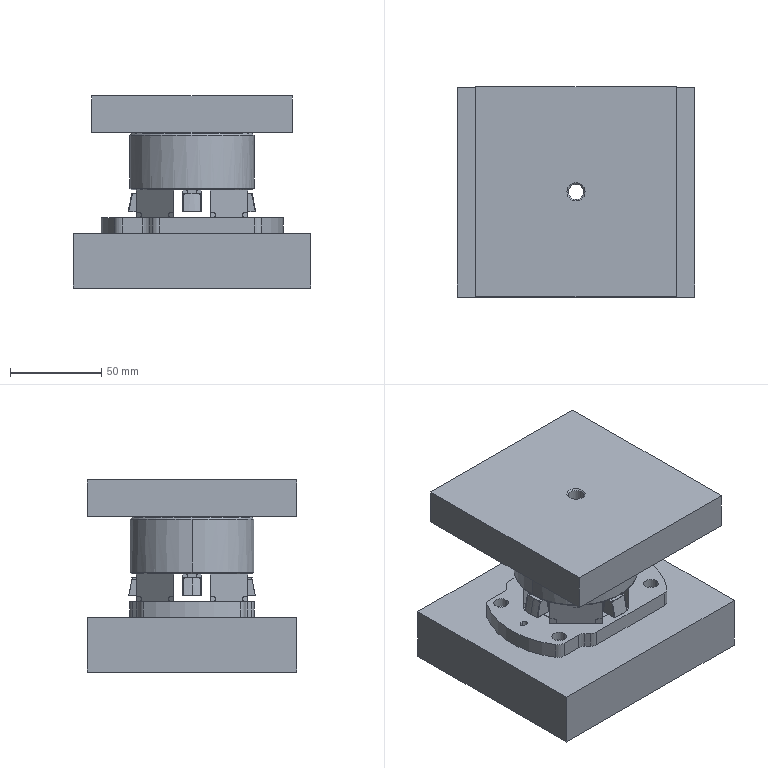CAM job | NX | 3+2 milling, drilling | part box 130 x 115 x 105.2 mm
Tools:
number,name,description,diameter,corner_radius,flute_length,length,flutes
12,ER16-D4-23,Milling Tool-5 Parameters,4.0,0.0,10.0,23.0,2
0,D1.5R0,Milling Tool-5 Parameters,1.5,0.0,50.0,75.0,2
20,D2,Milling Tool-5 Parameters,2.0,0.0,5.0,25.0,2
4,ER25-D10-50,Milling Tool-5 Parameters,10.0,0.0,20.0,50.0,2
11,ER25-D4-32,Milling Tool-5 Parameters,4.0,0.0,10.0,32.0,2
14,ER25-D2.5-23,Milling Tool-5 Parameters,2.5,0.0,0.0,10.0,2
16,ER25-D1.5-23,Milling Tool-5 Parameters,1.5,0.0,3.0,3.0,2
5,ER25-D10-50_G,Milling Tool-5 Parameters,10.0,0.0,20.0,50.0,2
12,ER25-D4-32_G,Milling Tool-5 Parameters,4.0,0.0,10.0,32.0,2
15,ER25-D2.5-23_G,Milling Tool-5 Parameters,2.5,0.0,10.0,10.0,2
17,ER25-D1.5-23_G,Milling Tool-5 Parameters,1.5,0.0,3.0,3.0,2
10,D8-55_PLUNGE,Milling Tool-5 Parameters,8.0,0.0,20.0,55.0,2
1,D50-120,Milling Tool-5 Parameters,50.0,0.0,5.0,120.0,2
3,D8.6,Drilling Tool,8.6,0.0,35.0,80.0,2
7,M4_D3.4,Drilling Tool,3.4,0.0,20.0,30.0,2
6,M10,Drilling Tool,8.6,0.0,35.0,40.0,2
8,M4,Drilling Tool,3.4,0.0,10.0,20.0,2
9,DRILL_D4.5,Drilling Tool,4.5,0.0,35.0,60.0,2
2,Φ10_CHAMFER,Chamfer Mill,10.0,0.0,20.0,55.0,2
Operations:
program,operation,operation_type,tool,method,geometry_group,spindle_rpm,surface_speed,feed_per_tooth,feed_cut,feed_plunge,cut_length_mm,path_length_mm,cut_time_min,machine_time_min
STEP1_FIXTURE,11,VolumeBased25DMillingOperation,D50-120,METHOD,MCS_1,3000.0,471.0,0.1667,1000.0,100.0,668.5,877.9,0.6685,0.6894
STEP1_FIXTURE,12,Operation,Φ10_CHAMFER,METHOD,MCS_1,2000.0,188.0,0.0125,100.0,100.0,16.0,462.529,0.16,0.2047
STEP1_FIXTURE,13,Operation,D8.6,METHOD,MCS_1,1400.0,37.0,0.0714,200.0,100.0,36.0,282.4,0.18,0.2046
STEP1_FIXTURE,14,PlanarMilling,ER25-D10-50,METHOD,MCS_1,5000.0,157.0,0.25,2500.0,100.0,538.082,793.482,0.2152,0.2564
STEP1_FIXTURE,HOLE_MILLING,CylinderMilling,ER25-D10-50,METHOD,MCS_1,5000.0,157.0,0.25,2500.0,100.0,1740.711,1985.911,0.6963,0.7358
STEP1_FIXTURE,15,PlanarMilling,ER25-D10-50_G,METHOD,MCS_1,5000.0,157.0,0.1,1000.0,100.0,534.941,790.341,0.5349,0.5761
STEP1_FIXTURE,HOLE_MILLING_COPY,CylinderMilling,ER25-D10-50_G,METHOD,MCS_1,5000.0,157.0,0.1,1000.0,100.0,353.731,601.61,0.3537,0.3938
STEP1_FIXTURE,16,Operation,M10,METHOD,MCS_1,100.0,2.0,0.75,150.0,100.0,26.0,297.4,0.1733,0.2005
STEP1_FIXTURE,17,Operation,M4_D3.4,METHOD,MCS_1,2000.0,188.0,0.0125,100.0,100.0,84.0,542.429,0.84,0.8858
STEP1_FIXTURE,18,Operation,M4,METHOD,MCS_1,200.0,2.0,0.35,140.0,100.0,64.0,515.488,0.4571,0.5023
STEP1_FIXTURE,PLANAR_TEXT,Engraving,Φ10_CHAMFER,METHOD,MCS_1,5000.0,157.0,0.1,1000.0,100.0,390.803,5495.523,0.3908,0.9013
STEP1_FIXTURE,PLANAR_MILL_1,PlanarMilling,Φ10_CHAMFER,METHOD,MCS_1,6500.0,204.0,0.0769,1000.0,100.0,208.638,422.038,0.2086,0.243
STEP1_FIXTURE,PLANAR_MILL_1_COPY,PlanarMilling,Φ10_CHAMFER,METHOD,MCS_1,6500.0,204.0,0.0769,1000.0,100.0,512.091,725.491,0.5121,0.5465
STEP1_FIXTURE,16_COPY,Operation,Φ10_CHAMFER,METHOD,MCS_1,2000.0,62.0,0.0375,150.0,100.0,6.0,257.4,0.04,0.0651
PROGRAM_1,DRILLING,Operation,Φ10_CHAMFER,METHOD,MCS_MILL,2000.0,62.0,0.0375,150.0,0.0,72.8,407.263,0.4853,0.5188
PROGRAM_1,110,Operation,DRILL_D4.5,METHOD,MCS_MILL,2000.0,188.0,0.0125,100.0,100.0,45.196,447.822,0.452,0.4922
PROGRAM_1,111,Operation,D8-55_PLUNGE,METHOD,MCS_MILL,1600.0,40.0,0.0625,200.0,100.0,24.0,405.429,0.12,0.1581
PROGRAM_1,112,PlanarMilling,ER25-D4-32,METHOD,MCS_MILL,5000.0,62.0,0.15,1500.0,100.0,1860.006,2853.586,1.24,1.397
PROGRAM_1,113,PlanarMilling,ER25-D4-32_G,METHOD,MCS_MILL,3500.0,43.0,0.0714,500.0,100.0,565.202,1104.256,1.393,1.475
PROGRAM_1,PLANAR_MILL,PlanarMilling,Φ10_CHAMFER,METHOD,MCS_MILL,3500.0,109.0,0.1429,1000.0,100.0,168.538,267.538,0.1685,0.1784
PROGRAM_1,PLANAR_MILL_COPY,PlanarMilling,Φ10_CHAMFER,METHOD,MCS_MILL,3500.0,109.0,0.0857,600.0,100.0,53.5,293.107,0.0892,0.1131
STEP2_FIXTURE,ADAPTIVE_MILLING_1,CavityMilling,ER25-D10-50,METHOD,MCS_2,6500.0,204.0,0.1923,2500.0,100.0,10997.187,11110.887,4.373,4.385
STEP2_FIXTURE,FLOOR_FACING,VolumeBased25DMillingOperation,ER25-D10-50_G,METHOD,MCS_2,6500.0,100.0,0.1178,800.0,100.0,1673.134,1787.134,2.091,2.103
STEP2_FIXTURE,116,Operation,Φ10_CHAMFER,METHOD,MCS_2,2000.0,188.0,0.0125,100.0,100.0,5.2,110.4,0.052,0.0625
STEP2_FIXTURE,117,Operation,D8.6,METHOD,MCS_2,2000.0,188.0,0.0125,100.0,100.0,23.483,146.965,0.2348,0.2472
STEP2_FIXTURE,118,Operation,M10,METHOD,MCS_2,100.0,2.0,0.75,150.0,100.0,11.0,122.0,0.0733,0.0844
STEP2_FIXTURE,121,PlanarMilling,ER16-D4-23,METHOD,MCS_2,5000.0,62.0,0.1,1000.0,100.0,808.881,954.35,0.8089,0.8324
STEP2_FIXTURE,123,PlanarMilling,Φ10_CHAMFER,METHOD,MCS_2,5000.0,157.0,0.1,1000.0,100.0,206.415,309.415,0.2306,0.2472
STEP2_FIXTURE,122,PlanarMilling,ER25-D4-32_G,METHOD,MCS_2,5000.0,62.0,0.1,1000.0,100.0,403.578,523.578,0.4229,0.4423
STEP2,125,PlanarMilling,ER25-D2.5-23,METHOD,MCS,6500.0,51.0,0.1154,1500.0,100.0,185.52,327.52,0.1237,0.146
STEP2,126,PlanarMilling,ER25-D2.5-23_G,METHOD,MCS,4934.0,31.0,0.0101,100.0,100.0,36.364,188.547,0.3636,0.3878
STEP2,ADAPTIVE_MILLING,CavityMilling,ER25-D10-50,METHOD,WORKPIECE_1,6500.0,204.0,0.1538,2000.0,100.0,4408.231,4554.231,1.344,1.358
STEP2,128,PlanarMilling,ER25-D10-50_G,METHOD,MCS,5000.0,157.0,0.1,1000.0,100.0,215.787,577.258,0.2158,0.2705
STEP2,128_COPY_1,PlanarMilling,ER25-D10-50_G,METHOD,MCS,5000.0,157.0,0.1,1000.0,100.0,215.42,576.784,0.226,0.2807
STEP2,128_COPY,PlanarMilling,Φ10_CHAMFER,METHOD,MCS,5000.0,157.0,0.1,1000.0,100.0,212.789,555.407,0.2128,0.2645
STEP2,129,Operation,Φ10_CHAMFER,METHOD,MCS,2000.0,188.0,0.0125,100.0,100.0,13.8,325.629,0.138,0.1692
STEP3_FIXTURE,FLOOR_WALL_1,VolumeBased25DMillingOperation,ER25-D10-50,METHOD,MCS_3,6500.0,204.0,0.1923,2500.0,100.0,6206.312,6861.071,2.482,2.548
STEP3_FIXTURE,130,CylinderMilling,ER25-D10-50,METHOD,MCS_3,6500.0,204.0,0.1923,2500.0,100.0,7743.479,7860.379,3.097,3.115
STEP3_FIXTURE,SPOT_FACING_2,Operation,Φ10_CHAMFER,METHOD,MCS_3,2000.0,188.0,0.0125,100.0,100.0,12.8,289.629,0.128,0.1557
STEP3_FIXTURE,PLANAR_MILL_1_4,PlanarMilling,Φ10_CHAMFER,METHOD,MCS_3,5000.0,157.0,0.1,1000.0,100.0,202.368,307.368,0.2024,0.2193
STEP3_FIXTURE,PLANAR_MILL_1_4_COPY,PlanarMilling,Φ10_CHAMFER,METHOD,MCS_3,5000.0,157.0,0.1,1000.0,100.0,40.38,136.38,0.0404,0.0558
STEP3_FIXTURE,131,PlanarMilling,Φ10_CHAMFER,METHOD,MCS_3,5000.0,157.0,0.1,1000.0,100.0,324.374,429.374,0.3244,0.3413
STEP3_FIXTURE,132,Operation,M4_D3.4,METHOD,MCS_3,2000.0,188.0,0.0125,100.0,100.0,84.0,432.029,0.84,0.8748
STEP3_FIXTURE,133,Operation,M4,METHOD,MCS_3,300.0,3.0,0.35,210.0,100.0,64.0,392.029,0.3048,0.3376
STEP3_FIXTURE,134,VolumeBased25DMillingOperation,ER25-D10-50_G,METHOD,MCS_3,5000.0,157.0,0.1,1000.0,100.0,70.481,169.482,0.0705,0.0804
STEP3_FIXTURE,HOLE_MILLING_1_COPY,CylinderMilling,ER25-D10-50_G,METHOD,MCS_3,5000.0,157.0,0.1,1000.0,100.0,353.812,491.288,0.3538,0.3761
STEP3_FIXTURE,FLOOR_WALL_1_COPY,VolumeBased25DMillingOperation,ER25-D10-50_G,METHOD,MCS_3,5000.0,157.0,0.1,1000.0,100.0,1126.923,1603.073,1.127,1.175
STEP3_4AXIS,135,PlanarMilling,ER25-D10-50,METHOD,MCS_4,5000.0,157.0,0.25,2500.0,100.0,649.504,815.238,0.2598,0.2863
STEP3_4AXIS,PLANAR_MILL_1_5_COPY,PlanarMilling,ER25-D10-50,METHOD,MCS_4,5000.0,157.0,0.25,2500.0,100.0,649.504,815.238,0.2598,0.2863
STEP3_4AXIS,PLANAR_MILL_1_5_COPY_1,PlanarMilling,ER25-D10-50,METHOD,MCS_4,5000.0,157.0,0.25,2500.0,100.0,649.504,815.238,0.2598,0.2863
STEP3_4AXIS,PLANAR_MILL_1_5_COPY_2,PlanarMilling,ER25-D10-50,METHOD,MCS_4,5000.0,157.0,0.25,2500.0,100.0,649.504,815.238,0.2598,0.2863
STEP3_4AXIS,136,PlanarMilling,ER25-D10-50_G,METHOD,MCS_4,5000.0,157.0,0.1,1000.0,100.0,93.186,235.683,0.0932,0.1161
STEP3_4AXIS,PLANAR_MILL_1_5_COPY_3_COPY,PlanarMilling,ER25-D10-50_G,METHOD,MCS_4,5000.0,157.0,0.1,1000.0,100.0,93.386,235.883,0.0934,0.1163
STEP3_4AXIS,PLANAR_MILL_1_5_COPY_3_COPY_1,PlanarMilling,ER25-D10-50_G,METHOD,MCS_4,5000.0,157.0,0.1,1000.0,100.0,93.386,235.883,0.0934,0.1163
STEP3_4AXIS,PLANAR_MILL_1_5_COPY_3_COPY_2,PlanarMilling,ER25-D10-50_G,METHOD,MCS_4,5000.0,157.0,0.1,1000.0,100.0,93.386,235.883,0.0934,0.1163
STEP3_4AXIS,137,PlanarMilling,ER25-D1.5-23,METHOD,MCS_4,5000.0,23.0,0.12,1200.0,100.0,650.732,755.682,0.5423,0.5589
STEP3_4AXIS,PLANAR_MILL_1_5_COPY_4_COPY_1,PlanarMilling,ER25-D1.5-23,METHOD,MCS_4,5000.0,23.0,0.12,1200.0,100.0,650.732,755.682,0.5423,0.5589
STEP3_4AXIS,PLANAR_MILL_1_5_COPY_4_COPY_2,PlanarMilling,ER25-D1.5-23,METHOD,MCS_4,5000.0,23.0,0.12,1200.0,100.0,650.732,755.682,0.5423,0.5589
STEP3_4AXIS,PLANAR_MILL_1_5_COPY_4_COPY_3,PlanarMilling,ER25-D1.5-23,METHOD,MCS_4,5000.0,23.0,0.12,1200.0,100.0,650.732,755.682,0.5423,0.5589
STEP3_4AXIS,VARIABLE_CONTOUR_COPY,SurfaceContour,Φ10_CHAMFER,METHOD,MCS_4_COPY,5000.0,157.0,0.1,1000.0,100.0,243.77,243.77,0.2438,0.2438
STEP3_4AXIS,VARIABLE_CONTOUR_COPY_COPY,SurfaceContour,Φ10_CHAMFER,METHOD,MCS_4_COPY,5000.0,157.0,0.1,1000.0,100.0,244.183,244.183,0.2442,0.2442
STEP3_4AXIS,PLANAR_MILL_1_1,PlanarMilling,ER25-D2.5-23,METHOD,MCS_4,6500.0,51.0,0.0769,1000.0,100.0,200.658,328.017,0.2007,0.2206
STEP3_4AXIS,PLANAR_MILL_1_1_COPY,PlanarMilling,ER25-D2.5-23,METHOD,MCS_4,6500.0,51.0,0.0769,1000.0,100.0,200.658,328.017,0.2007,0.2206
STEP3_4AXIS,PLANAR_MILL_1_1_COPY_3_COPY_1,PlanarMilling,ER25-D2.5-23,METHOD,MCS_4,6500.0,51.0,0.1077,1400.0,100.0,200.658,328.017,0.1433,0.1633
STEP3_4AXIS,PLANAR_MILL_1_1_COPY_3_COPY_2,PlanarMilling,ER25-D2.5-23,METHOD,MCS_4,6500.0,51.0,0.1077,1400.0,100.0,200.658,328.017,0.1433,0.1633
STEP3_4AXIS,138,PlanarMilling,ER25-D1.5-23_G,METHOD,MCS_4,5000.0,23.0,0.03,300.0,100.0,80.507,191.709,0.2684,0.2861
STEP3_4AXIS,PLANAR_MILL_1_5_COPY_4_COPY_COPY,PlanarMilling,ER25-D1.5-23_G,METHOD,MCS_4,5000.0,23.0,0.03,300.0,100.0,80.807,192.008,0.2694,0.2871
STEP3_4AXIS,PLANAR_MILL_1_5_COPY_4_COPY_COPY_1,PlanarMilling,ER25-D1.5-23_G,METHOD,MCS_4,5000.0,23.0,0.03,300.0,100.0,80.807,192.008,0.2694,0.2871
STEP3_4AXIS,PLANAR_MILL_1_5_COPY_4_COPY_COPY_2,PlanarMilling,ER25-D1.5-23_G,METHOD,MCS_4,5000.0,23.0,0.03,300.0,100.0,80.807,192.008,0.2694,0.2871
EXTRA_MACHINING1,PLANAR_MILL_COPY_4,PlanarMilling,D1.5R0,METHOD,MCS_4_COPY,6000.0,0.0,0.1364,1400.0,100.0,1053.834,2900.619,0.7527,0.9909
EXTRA_MACHINING1,PLANAR_MILL_COPY_4_COPY,PlanarMilling,D1.5R0,METHOD,MCS_4_COPY,6000.0,0.0,0.1364,1400.0,100.0,1053.834,2900.619,0.7527,0.9909
EXTRA_MACHINING1,PLANAR_MILL_COPY_4_COPY_1,PlanarMilling,D1.5R0,METHOD,MCS_4_COPY,6000.0,0.0,0.1364,1400.0,100.0,1053.834,2900.619,0.7527,0.9909
EXTRA_MACHINING1,PLANAR_MILL_COPY_4_COPY_2,PlanarMilling,D1.5R0,METHOD,MCS_4_COPY,6000.0,0.0,0.1364,1400.0,100.0,1053.834,2900.619,0.7527,0.9909
PROGRAM_2,PLANAR_MILL_COPY_4_COPY_3_COPY_1,PlanarMilling,D2,METHOD,MCS_4_COPY,6000.0,0.0,0.1364,1200.0,100.0,391.397,579.539,0.3262,0.3505
PROGRAM_2,PLANAR_MILL_COPY_4_COPY_3_COPY_1_COPY,PlanarMilling,D2,METHOD,MCS_4_COPY,6000.0,0.0,0.1364,1200.0,100.0,391.397,579.539,0.3262,0.3505
PROGRAM_2,PLANAR_MILL_COPY_4_COPY_3_COPY_1_COPY_1,PlanarMilling,D2,METHOD,MCS_4_COPY,6000.0,0.0,0.1364,1200.0,100.0,391.397,579.539,0.3262,0.3505
PROGRAM_2,PLANAR_MILL_COPY_4_COPY_3_COPY_1_COPY_2,PlanarMilling,D2,METHOD,MCS_4_COPY,6000.0,0.0,0.1364,1200.0,100.0,391.397,579.539,0.3262,0.3505